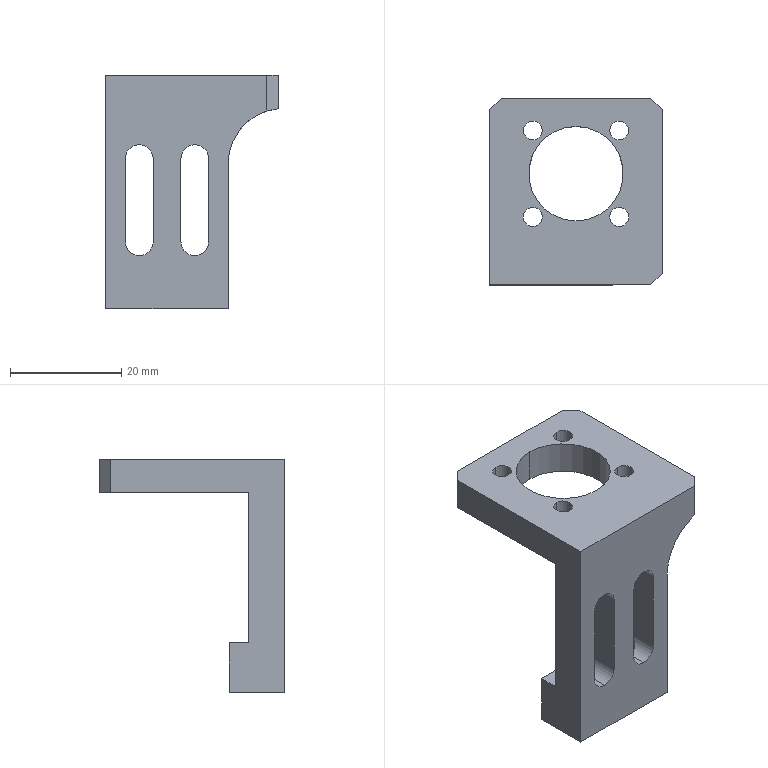Part | 1 solid | 39 faces | box 31 x 33.478 x 42 mm | volume 9262 mm3 | cylinder 21 | plane 18 | commonest cylinder face diameters 3.4 x8 5 x6 2.5 x4 17 x2 20 x1
STEP:
#1=CARTESIAN_POINT('',(7.778,9.339,0.));
#2=VERTEX_POINT('',#1);
#3=CARTESIAN_POINT('',(7.778,12.739,0.));
#4=VERTEX_POINT('',#3);
#5=CARTESIAN_POINT('',(7.778,11.039,0.));
#6=DIRECTION('',(0.,0.,-1.));
#7=DIRECTION('',(0.,1.,0.));
#8=AXIS2_PLACEMENT_3D('',#5,#6,#7);
#9=CIRCLE('',#8,1.7);
#10=EDGE_CURVE('',#2,#4,#9,.T.);
#11=ORIENTED_EDGE('',*,*,#10,.F.);
#12=CARTESIAN_POINT('',(7.778,9.339,-6.));
#13=VERTEX_POINT('',#12);
#14=CARTESIAN_POINT('',(7.778,9.339,-6.));
#15=DIRECTION('',(0.,0.,-1.));
#16=VECTOR('',#15,1000.);
#17=LINE('',#14,#16);
#18=EDGE_CURVE('',#13,#2,#17,.F.);
#19=ORIENTED_EDGE('',*,*,#18,.F.);
#20=CARTESIAN_POINT('',(7.778,12.739,-6.));
#21=VERTEX_POINT('',#20);
#22=CARTESIAN_POINT('',(7.778,11.039,-6.));
#23=DIRECTION('',(0.,0.,-1.));
#24=DIRECTION('',(0.,1.,0.));
#25=AXIS2_PLACEMENT_3D('',#22,#23,#24);
#26=CIRCLE('',#25,1.7);
#27=EDGE_CURVE('',#13,#21,#26,.T.);
#28=ORIENTED_EDGE('',*,*,#27,.T.);
#29=CARTESIAN_POINT('',(7.778,12.739,-6.));
#30=DIRECTION('',(0.,0.,-1.));
#31=VECTOR('',#30,1000.);
#32=LINE('',#29,#31);
#33=EDGE_CURVE('',#21,#4,#32,.F.);
#34=ORIENTED_EDGE('',*,*,#33,.T.);
#35=EDGE_LOOP('',(#11,#19,#28,#34));
#36=FACE_BOUND('',#35,.T.);
#37=CARTESIAN_POINT('',(7.778,11.039,-6.));
#38=DIRECTION('',(0.,0.,-1.));
#39=DIRECTION('',(0.,-1.,0.));
#40=AXIS2_PLACEMENT_3D('',#37,#38,#39);
#41=CYLINDRICAL_SURFACE('',#40,1.7);
#42=ADVANCED_FACE('',(#36),#41,.F.);
#43=CARTESIAN_POINT('',(7.778,-6.217,0.));
#44=VERTEX_POINT('',#43);
#45=CARTESIAN_POINT('',(7.778,-2.817,0.));
#46=VERTEX_POINT('',#45);
#47=CARTESIAN_POINT('',(7.778,-4.517,0.));
#48=DIRECTION('',(0.,0.,-1.));
#49=DIRECTION('',(0.,1.,0.));
#50=AXIS2_PLACEMENT_3D('',#47,#48,#49);
#51=CIRCLE('',#50,1.7);
#52=EDGE_CURVE('',#44,#46,#51,.T.);
#53=ORIENTED_EDGE('',*,*,#52,.F.);
#54=CARTESIAN_POINT('',(7.778,-6.217,-6.));
#55=VERTEX_POINT('',#54);
#56=CARTESIAN_POINT('',(7.778,-6.217,-6.));
#57=DIRECTION('',(0.,0.,-1.));
#58=VECTOR('',#57,1000.);
#59=LINE('',#56,#58);
#60=EDGE_CURVE('',#55,#44,#59,.F.);
#61=ORIENTED_EDGE('',*,*,#60,.F.);
#62=CARTESIAN_POINT('',(7.778,-2.817,-6.));
#63=VERTEX_POINT('',#62);
#64=CARTESIAN_POINT('',(7.778,-4.517,-6.));
#65=DIRECTION('',(0.,0.,-1.));
#66=DIRECTION('',(0.,1.,0.));
#67=AXIS2_PLACEMENT_3D('',#64,#65,#66);
#68=CIRCLE('',#67,1.7);
#69=EDGE_CURVE('',#55,#63,#68,.T.);
#70=ORIENTED_EDGE('',*,*,#69,.T.);
#71=CARTESIAN_POINT('',(7.778,-2.817,-6.));
#72=DIRECTION('',(0.,0.,-1.));
#73=VECTOR('',#72,1000.);
#74=LINE('',#71,#73);
#75=EDGE_CURVE('',#63,#46,#74,.F.);
#76=ORIENTED_EDGE('',*,*,#75,.T.);
#77=EDGE_LOOP('',(#53,#61,#70,#76));
#78=FACE_BOUND('',#77,.T.);
#79=CARTESIAN_POINT('',(7.778,-4.517,-6.));
#80=DIRECTION('',(0.,0.,-1.));
#81=DIRECTION('',(0.,-1.,0.));
#82=AXIS2_PLACEMENT_3D('',#79,#80,#81);
#83=CYLINDRICAL_SURFACE('',#82,1.7);
#84=ADVANCED_FACE('',(#78),#83,.F.);
#85=CARTESIAN_POINT('',(-7.778,9.339,0.));
#86=VERTEX_POINT('',#85);
#87=CARTESIAN_POINT('',(-7.778,12.739,0.));
#88=VERTEX_POINT('',#87);
#89=CARTESIAN_POINT('',(-7.778,11.039,0.));
#90=DIRECTION('',(0.,0.,-1.));
#91=DIRECTION('',(0.,1.,0.));
#92=AXIS2_PLACEMENT_3D('',#89,#90,#91);
#93=CIRCLE('',#92,1.7);
#94=EDGE_CURVE('',#86,#88,#93,.T.);
#95=ORIENTED_EDGE('',*,*,#94,.F.);
#96=CARTESIAN_POINT('',(-7.778,9.339,-6.));
#97=VERTEX_POINT('',#96);
#98=CARTESIAN_POINT('',(-7.778,9.339,-6.));
#99=DIRECTION('',(0.,0.,-1.));
#100=VECTOR('',#99,1000.);
#101=LINE('',#98,#100);
#102=EDGE_CURVE('',#97,#86,#101,.F.);
#103=ORIENTED_EDGE('',*,*,#102,.F.);
#104=CARTESIAN_POINT('',(-7.778,12.739,-6.));
#105=VERTEX_POINT('',#104);
#106=CARTESIAN_POINT('',(-7.778,11.039,-6.));
#107=DIRECTION('',(0.,0.,-1.));
#108=DIRECTION('',(0.,1.,0.));
#109=AXIS2_PLACEMENT_3D('',#106,#107,#108);
#110=CIRCLE('',#109,1.7);
#111=EDGE_CURVE('',#97,#105,#110,.T.);
#112=ORIENTED_EDGE('',*,*,#111,.T.);
#113=CARTESIAN_POINT('',(-7.778,12.739,-6.));
#114=DIRECTION('',(0.,0.,-1.));
#115=VECTOR('',#114,1000.);
#116=LINE('',#113,#115);
#117=EDGE_CURVE('',#105,#88,#116,.F.);
#118=ORIENTED_EDGE('',*,*,#117,.T.);
#119=EDGE_LOOP('',(#95,#103,#112,#118));
#120=FACE_BOUND('',#119,.T.);
#121=CARTESIAN_POINT('',(-7.778,11.039,-6.));
#122=DIRECTION('',(0.,0.,-1.));
#123=DIRECTION('',(0.,-1.,0.));
#124=AXIS2_PLACEMENT_3D('',#121,#122,#123);
#125=CYLINDRICAL_SURFACE('',#124,1.7);
#126=ADVANCED_FACE('',(#120),#125,.F.);
#127=CARTESIAN_POINT('',(-7.778,-6.217,0.));
#128=VERTEX_POINT('',#127);
#129=CARTESIAN_POINT('',(-7.778,-2.817,0.));
#130=VERTEX_POINT('',#129);
#131=CARTESIAN_POINT('',(-7.778,-4.517,0.));
#132=DIRECTION('',(0.,0.,-1.));
#133=DIRECTION('',(0.,1.,0.));
#134=AXIS2_PLACEMENT_3D('',#131,#132,#133);
#135=CIRCLE('',#134,1.7);
#136=EDGE_CURVE('',#128,#130,#135,.T.);
#137=ORIENTED_EDGE('',*,*,#136,.F.);
#138=CARTESIAN_POINT('',(-7.778,-6.217,-6.));
#139=VERTEX_POINT('',#138);
#140=CARTESIAN_POINT('',(-7.778,-6.217,-6.));
#141=DIRECTION('',(0.,0.,-1.));
#142=VECTOR('',#141,1000.);
#143=LINE('',#140,#142);
#144=EDGE_CURVE('',#139,#128,#143,.F.);
#145=ORIENTED_EDGE('',*,*,#144,.F.);
#146=CARTESIAN_POINT('',(-7.778,-2.817,-6.));
#147=VERTEX_POINT('',#146);
#148=CARTESIAN_POINT('',(-7.778,-4.517,-6.));
#149=DIRECTION('',(0.,0.,-1.));
#150=DIRECTION('',(0.,1.,0.));
#151=AXIS2_PLACEMENT_3D('',#148,#149,#150);
#152=CIRCLE('',#151,1.7);
#153=EDGE_CURVE('',#139,#147,#152,.T.);
#154=ORIENTED_EDGE('',*,*,#153,.T.);
#155=CARTESIAN_POINT('',(-7.778,-2.817,-6.));
#156=DIRECTION('',(0.,0.,-1.));
#157=VECTOR('',#156,1000.);
#158=LINE('',#155,#157);
#159=EDGE_CURVE('',#147,#130,#158,.F.);
#160=ORIENTED_EDGE('',*,*,#159,.T.);
#161=EDGE_LOOP('',(#137,#145,#154,#160));
#162=FACE_BOUND('',#161,.T.);
#163=CARTESIAN_POINT('',(-7.778,-4.517,-6.));
#164=DIRECTION('',(0.,0.,-1.));
#165=DIRECTION('',(0.,-1.,0.));
#166=AXIS2_PLACEMENT_3D('',#163,#164,#165);
#167=CYLINDRICAL_SURFACE('',#166,1.7);
#168=ADVANCED_FACE('',(#162),#167,.F.);
#169=CARTESIAN_POINT('',(0.,-5.239,-6.));
#170=VERTEX_POINT('',#169);
#171=CARTESIAN_POINT('',(0.,11.761,-6.));
#172=VERTEX_POINT('',#171);
#173=CARTESIAN_POINT('',(0.,3.261,-6.));
#174=DIRECTION('',(0.,0.,-1.));
#175=DIRECTION('',(0.,1.,0.));
#176=AXIS2_PLACEMENT_3D('',#173,#174,#175);
#177=CIRCLE('',#176,8.5);
#178=EDGE_CURVE('',#170,#172,#177,.T.);
#179=ORIENTED_EDGE('',*,*,#178,.T.);
#180=CARTESIAN_POINT('',(0.,11.761,0.));
#181=VERTEX_POINT('',#180);
#182=CARTESIAN_POINT('',(0.,11.761,-42.));
#183=DIRECTION('',(0.,0.,1.));
#184=VECTOR('',#183,1000.);
#185=LINE('',#182,#184);
#186=EDGE_CURVE('',#181,#172,#185,.F.);
#187=ORIENTED_EDGE('',*,*,#186,.F.);
#188=CARTESIAN_POINT('',(0.,-5.239,0.));
#189=VERTEX_POINT('',#188);
#190=CARTESIAN_POINT('',(0.,3.261,0.));
#191=DIRECTION('',(0.,0.,1.));
#192=DIRECTION('',(0.,-1.,0.));
#193=AXIS2_PLACEMENT_3D('',#190,#191,#192);
#194=CIRCLE('',#193,8.5);
#195=EDGE_CURVE('',#181,#189,#194,.T.);
#196=ORIENTED_EDGE('',*,*,#195,.T.);
#197=CARTESIAN_POINT('',(0.,-5.239,-42.));
#198=DIRECTION('',(0.,0.,1.));
#199=VECTOR('',#198,1000.);
#200=LINE('',#197,#199);
#201=EDGE_CURVE('',#189,#170,#200,.F.);
#202=ORIENTED_EDGE('',*,*,#201,.T.);
#203=EDGE_LOOP('',(#179,#187,#196,#202));
#204=FACE_BOUND('',#203,.T.);
#205=CARTESIAN_POINT('',(0.,3.261,-42.));
#206=DIRECTION('',(0.,0.,1.));
#207=DIRECTION('',(0.,1.,0.));
#208=AXIS2_PLACEMENT_3D('',#205,#206,#207);
#209=CYLINDRICAL_SURFACE('',#208,8.5);
#210=ADVANCED_FACE('',(#204),#209,.F.);
#211=CARTESIAN_POINT('',(-7.,-10.239,-30.));
#212=VERTEX_POINT('',#211);
#213=CARTESIAN_POINT('',(-9.5,-10.239,-32.5));
#214=VERTEX_POINT('',#213);
#215=CARTESIAN_POINT('',(-9.5,-10.239,-30.));
#216=DIRECTION('',(0.,1.,0.));
#217=DIRECTION('',(0.,0.,-1.));
#218=AXIS2_PLACEMENT_3D('',#215,#216,#217);
#219=CIRCLE('',#218,2.5);
#220=EDGE_CURVE('',#212,#214,#219,.T.);
#221=ORIENTED_EDGE('',*,*,#220,.T.);
#222=CARTESIAN_POINT('',(-9.5,-10.989,-32.5));
#223=VERTEX_POINT('',#222);
#224=CARTESIAN_POINT('',(-9.5,25.261,-32.5));
#225=DIRECTION('',(0.,-1.,0.));
#226=VECTOR('',#225,1000.);
#227=LINE('',#224,#226);
#228=EDGE_CURVE('',#214,#223,#227,.T.);
#229=ORIENTED_EDGE('',*,*,#228,.T.);
#230=CARTESIAN_POINT('',(-9.5,-12.489,-32.5));
#231=VERTEX_POINT('',#230);
#232=CARTESIAN_POINT('',(-9.5,-12.489,-32.5));
#233=CARTESIAN_POINT('',(-9.175,-12.056,-32.5));
#234=CARTESIAN_POINT('',(-9.175,-11.422,-32.5));
#235=CARTESIAN_POINT('',(-9.5,-10.989,-32.5));
#236=B_SPLINE_CURVE_WITH_KNOTS('',3,(#232,#233,#234,#235),.UNSPECIFIED.,.F.,.F.,(4,4),(0.,0.0016),.UNSPECIFIED.);
#237=EDGE_CURVE('',#231,#223,#236,.T.);
#238=ORIENTED_EDGE('',*,*,#237,.F.);
#239=CARTESIAN_POINT('',(-9.5,-16.739,-32.5));
#240=VERTEX_POINT('',#239);
#241=CARTESIAN_POINT('',(-9.5,25.261,-32.5));
#242=DIRECTION('',(0.,-1.,0.));
#243=VECTOR('',#242,1000.);
#244=LINE('',#241,#243);
#245=EDGE_CURVE('',#231,#240,#244,.T.);
#246=ORIENTED_EDGE('',*,*,#245,.T.);
#247=CARTESIAN_POINT('',(-7.,-16.739,-30.));
#248=VERTEX_POINT('',#247);
#249=CARTESIAN_POINT('',(-9.5,-16.739,-30.));
#250=DIRECTION('',(0.,-1.,0.));
#251=DIRECTION('',(0.,0.,-1.));
#252=AXIS2_PLACEMENT_3D('',#249,#250,#251);
#253=CIRCLE('',#252,2.5);
#254=EDGE_CURVE('',#240,#248,#253,.T.);
#255=ORIENTED_EDGE('',*,*,#254,.T.);
#256=CARTESIAN_POINT('',(-7.,25.261,-30.));
#257=DIRECTION('',(0.,-1.,0.));
#258=VECTOR('',#257,1000.);
#259=LINE('',#256,#258);
#260=EDGE_CURVE('',#212,#248,#259,.T.);
#261=ORIENTED_EDGE('',*,*,#260,.F.);
#262=EDGE_LOOP('',(#221,#229,#238,#246,#255,#261));
#263=FACE_BOUND('',#262,.T.);
#264=CARTESIAN_POINT('',(-9.5,25.261,-30.));
#265=DIRECTION('',(0.,-1.,0.));
#266=DIRECTION('',(0.,0.,1.));
#267=AXIS2_PLACEMENT_3D('',#264,#265,#266);
#268=CYLINDRICAL_SURFACE('',#267,2.5);
#269=ADVANCED_FACE('',(#263),#268,.F.);
#270=CARTESIAN_POINT('',(3.,-10.239,-30.));
#271=VERTEX_POINT('',#270);
#272=CARTESIAN_POINT('',(0.5,-10.239,-32.5));
#273=VERTEX_POINT('',#272);
#274=CARTESIAN_POINT('',(0.5,-10.239,-30.));
#275=DIRECTION('',(0.,1.,0.));
#276=DIRECTION('',(0.,0.,-1.));
#277=AXIS2_PLACEMENT_3D('',#274,#275,#276);
#278=CIRCLE('',#277,2.5);
#279=EDGE_CURVE('',#271,#273,#278,.T.);
#280=ORIENTED_EDGE('',*,*,#279,.T.);
#281=CARTESIAN_POINT('',(0.5,-10.989,-32.5));
#282=VERTEX_POINT('',#281);
#283=CARTESIAN_POINT('',(0.5,25.261,-32.5));
#284=DIRECTION('',(0.,-1.,0.));
#285=VECTOR('',#284,1000.);
#286=LINE('',#283,#285);
#287=EDGE_CURVE('',#273,#282,#286,.T.);
#288=ORIENTED_EDGE('',*,*,#287,.T.);
#289=CARTESIAN_POINT('',(1.5,-10.489,-32.291));
#290=VERTEX_POINT('',#289);
#291=CARTESIAN_POINT('',(1.5,-10.489,-32.291));
#292=CARTESIAN_POINT('',(1.134,-10.489,-32.451));
#293=CARTESIAN_POINT('',(0.7396,-10.67,-32.5));
#294=CARTESIAN_POINT('',(0.5,-10.989,-32.5));
#295=B_SPLINE_CURVE_WITH_KNOTS('',3,(#291,#292,#293,#294),.UNSPECIFIED.,.F.,.F.,(4,4),(0.,0.001181),.UNSPECIFIED.);
#296=EDGE_CURVE('',#290,#282,#295,.T.);
#297=ORIENTED_EDGE('',*,*,#296,.F.);
#298=CARTESIAN_POINT('',(1.5,-12.989,-32.291));
#299=VERTEX_POINT('',#298);
#300=CARTESIAN_POINT('',(1.5,-12.989,-32.291));
#301=CARTESIAN_POINT('',(1.859,-12.989,-32.134));
#302=CARTESIAN_POINT('',(2.307,-12.765,-31.78));
#303=CARTESIAN_POINT('',(2.657,-12.293,-31.285));
#304=CARTESIAN_POINT('',(2.796,-11.741,-30.992));
#305=CARTESIAN_POINT('',(2.658,-11.187,-31.284));
#306=CARTESIAN_POINT('',(2.309,-10.714,-31.779));
#307=CARTESIAN_POINT('',(1.859,-10.489,-32.135));
#308=CARTESIAN_POINT('',(1.5,-10.489,-32.291));
#309=B_SPLINE_CURVE_WITH_KNOTS('',3,(#300,#301,#302,#303,#304,#305,#306,#307,#308),.UNSPECIFIED.,.F.,.F.,(4,1,1,1,1,1,4),(0.,0.001157,0.001735,0.002314,0.002892,0.003471,0.004627),.UNSPECIFIED.);
#310=EDGE_CURVE('',#299,#290,#309,.T.);
#311=ORIENTED_EDGE('',*,*,#310,.F.);
#312=CARTESIAN_POINT('',(0.5,-12.489,-32.5));
#313=VERTEX_POINT('',#312);
#314=CARTESIAN_POINT('',(0.5,-12.489,-32.5));
#315=CARTESIAN_POINT('',(0.7395,-12.808,-32.5));
#316=CARTESIAN_POINT('',(1.134,-12.989,-32.451));
#317=CARTESIAN_POINT('',(1.5,-12.989,-32.291));
#318=B_SPLINE_CURVE_WITH_KNOTS('',3,(#314,#315,#316,#317),.UNSPECIFIED.,.F.,.F.,(4,4),(0.,0.001181),.UNSPECIFIED.);
#319=EDGE_CURVE('',#313,#299,#318,.T.);
#320=ORIENTED_EDGE('',*,*,#319,.F.);
#321=CARTESIAN_POINT('',(0.5,-16.739,-32.5));
#322=VERTEX_POINT('',#321);
#323=CARTESIAN_POINT('',(0.5,25.261,-32.5));
#324=DIRECTION('',(0.,-1.,0.));
#325=VECTOR('',#324,1000.);
#326=LINE('',#323,#325);
#327=EDGE_CURVE('',#313,#322,#326,.T.);
#328=ORIENTED_EDGE('',*,*,#327,.T.);
#329=CARTESIAN_POINT('',(3.,-16.739,-30.));
#330=VERTEX_POINT('',#329);
#331=CARTESIAN_POINT('',(0.5,-16.739,-30.));
#332=DIRECTION('',(0.,-1.,0.));
#333=DIRECTION('',(0.,0.,-1.));
#334=AXIS2_PLACEMENT_3D('',#331,#332,#333);
#335=CIRCLE('',#334,2.5);
#336=EDGE_CURVE('',#322,#330,#335,.T.);
#337=ORIENTED_EDGE('',*,*,#336,.T.);
#338=CARTESIAN_POINT('',(3.,25.261,-30.));
#339=DIRECTION('',(0.,-1.,0.));
#340=VECTOR('',#339,1000.);
#341=LINE('',#338,#340);
#342=EDGE_CURVE('',#271,#330,#341,.T.);
#343=ORIENTED_EDGE('',*,*,#342,.F.);
#344=EDGE_LOOP('',(#280,#288,#297,#311,#320,#328,#337,#343));
#345=FACE_BOUND('',#344,.T.);
#346=CARTESIAN_POINT('',(0.5,25.261,-30.));
#347=DIRECTION('',(0.,-1.,0.));
#348=DIRECTION('',(0.,0.,1.));
#349=AXIS2_PLACEMENT_3D('',#346,#347,#348);
#350=CYLINDRICAL_SURFACE('',#349,2.5);
#351=ADVANCED_FACE('',(#345),#350,.F.);
#352=ORIENTED_EDGE('',*,*,#296,.T.);
#353=CARTESIAN_POINT('',(0.5,-10.989,-32.5));
#354=CARTESIAN_POINT('',(0.1753,-11.422,-32.5));
#355=CARTESIAN_POINT('',(0.1753,-12.056,-32.5));
#356=CARTESIAN_POINT('',(0.5,-12.489,-32.5));
#357=B_SPLINE_CURVE_WITH_KNOTS('',3,(#353,#354,#355,#356),.UNSPECIFIED.,.F.,.F.,(4,4),(0.,0.0016),.UNSPECIFIED.);
#358=EDGE_CURVE('',#282,#313,#357,.T.);
#359=ORIENTED_EDGE('',*,*,#358,.T.);
#360=ORIENTED_EDGE('',*,*,#319,.T.);
#361=CARTESIAN_POINT('',(1.5,-12.989,-42.));
#362=VERTEX_POINT('',#361);
#363=CARTESIAN_POINT('',(1.5,-12.989,-42.));
#364=DIRECTION('',(0.,0.,-1.));
#365=VECTOR('',#364,1000.);
#366=LINE('',#363,#365);
#367=EDGE_CURVE('',#362,#299,#366,.F.);
#368=ORIENTED_EDGE('',*,*,#367,.F.);
#369=CARTESIAN_POINT('',(1.5,-10.489,-42.));
#370=VERTEX_POINT('',#369);
#371=CARTESIAN_POINT('',(1.5,-11.739,-42.));
#372=DIRECTION('',(0.,0.,-1.));
#373=DIRECTION('',(0.,1.,0.));
#374=AXIS2_PLACEMENT_3D('',#371,#372,#373);
#375=CIRCLE('',#374,1.25);
#376=EDGE_CURVE('',#362,#370,#375,.T.);
#377=ORIENTED_EDGE('',*,*,#376,.T.);
#378=CARTESIAN_POINT('',(1.5,-10.489,-42.));
#379=DIRECTION('',(0.,0.,-1.));
#380=VECTOR('',#379,1000.);
#381=LINE('',#378,#380);
#382=EDGE_CURVE('',#370,#290,#381,.F.);
#383=ORIENTED_EDGE('',*,*,#382,.T.);
#384=EDGE_LOOP('',(#352,#359,#360,#368,#377,#383));
#385=FACE_BOUND('',#384,.T.);
#386=CARTESIAN_POINT('',(1.5,-11.739,-42.));
#387=DIRECTION('',(0.,0.,-1.));
#388=DIRECTION('',(0.,-1.,0.));
#389=AXIS2_PLACEMENT_3D('',#386,#387,#388);
#390=CYLINDRICAL_SURFACE('',#389,1.25);
#391=ADVANCED_FACE('',(#385),#390,.F.);
#392=CARTESIAN_POINT('',(-10.5,-10.489,-32.291));
#393=VERTEX_POINT('',#392);
#394=CARTESIAN_POINT('',(-10.5,-12.989,-32.291));
#395=VERTEX_POINT('',#394);
#396=CARTESIAN_POINT('',(-10.5,-10.489,-32.291));
#397=CARTESIAN_POINT('',(-10.859,-10.489,-32.134));
#398=CARTESIAN_POINT('',(-11.307,-10.713,-31.78));
#399=CARTESIAN_POINT('',(-11.657,-11.185,-31.285));
#400=CARTESIAN_POINT('',(-11.796,-11.738,-30.992));
#401=CARTESIAN_POINT('',(-11.658,-12.291,-31.284));
#402=CARTESIAN_POINT('',(-11.309,-12.764,-31.779));
#403=CARTESIAN_POINT('',(-10.859,-12.989,-32.135));
#404=CARTESIAN_POINT('',(-10.5,-12.989,-32.291));
#405=B_SPLINE_CURVE_WITH_KNOTS('',3,(#396,#397,#398,#399,#400,#401,#402,#403,#404),.UNSPECIFIED.,.F.,.F.,(4,1,1,1,1,1,4),(0.,0.001157,0.001735,0.002314,0.002892,0.003471,0.004627),.UNSPECIFIED.);
#406=EDGE_CURVE('',#393,#395,#405,.T.);
#407=ORIENTED_EDGE('',*,*,#406,.T.);
#408=CARTESIAN_POINT('',(-10.5,-12.989,-42.));
#409=VERTEX_POINT('',#408);
#410=CARTESIAN_POINT('',(-10.5,-12.989,-42.));
#411=DIRECTION('',(0.,0.,-1.));
#412=VECTOR('',#411,1000.);
#413=LINE('',#410,#412);
#414=EDGE_CURVE('',#409,#395,#413,.F.);
#415=ORIENTED_EDGE('',*,*,#414,.F.);
#416=CARTESIAN_POINT('',(-10.5,-10.489,-42.));
#417=VERTEX_POINT('',#416);
#418=CARTESIAN_POINT('',(-10.5,-11.739,-42.));
#419=DIRECTION('',(0.,0.,-1.));
#420=DIRECTION('',(0.,1.,0.));
#421=AXIS2_PLACEMENT_3D('',#418,#419,#420);
#422=CIRCLE('',#421,1.25);
#423=EDGE_CURVE('',#409,#417,#422,.T.);
#424=ORIENTED_EDGE('',*,*,#423,.T.);
#425=CARTESIAN_POINT('',(-10.5,-10.489,-42.));
#426=DIRECTION('',(0.,0.,-1.));
#427=VECTOR('',#426,1000.);
#428=LINE('',#425,#427);
#429=EDGE_CURVE('',#417,#393,#428,.F.);
#430=ORIENTED_EDGE('',*,*,#429,.T.);
#431=EDGE_LOOP('',(#407,#415,#424,#430));
#432=FACE_BOUND('',#431,.T.);
#433=CARTESIAN_POINT('',(-10.5,-11.739,-42.));
#434=DIRECTION('',(0.,0.,-1.));
#435=DIRECTION('',(0.,-1.,0.));
#436=AXIS2_PLACEMENT_3D('',#433,#434,#435);
#437=CYLINDRICAL_SURFACE('',#436,1.25);
#438=ADVANCED_FACE('',(#432),#437,.F.);
#439=CARTESIAN_POINT('',(15.5,-14.739,0.));
#440=VERTEX_POINT('',#439);
#441=CARTESIAN_POINT('',(15.5,14.739,0.));
#442=VERTEX_POINT('',#441);
#443=CARTESIAN_POINT('',(15.5,25.261,0.));
#444=DIRECTION('',(0.,1.,0.));
#445=VECTOR('',#444,1000.);
#446=LINE('',#443,#445);
#447=EDGE_CURVE('',#440,#442,#446,.T.);
#448=ORIENTED_EDGE('',*,*,#447,.F.);
#449=CARTESIAN_POINT('',(15.5,-14.739,-6.));
#450=VERTEX_POINT('',#449);
#451=CARTESIAN_POINT('',(15.5,-14.739,-6.));
#452=DIRECTION('',(0.,0.,-1.));
#453=VECTOR('',#452,1000.);
#454=LINE('',#451,#453);
#455=EDGE_CURVE('',#440,#450,#454,.T.);
#456=ORIENTED_EDGE('',*,*,#455,.T.);
#457=CARTESIAN_POINT('',(15.5,-10.239,-6.));
#458=VERTEX_POINT('',#457);
#459=CARTESIAN_POINT('',(15.5,25.261,-6.));
#460=DIRECTION('',(0.,1.,0.));
#461=VECTOR('',#460,1000.);
#462=LINE('',#459,#461);
#463=EDGE_CURVE('',#450,#458,#462,.T.);
#464=ORIENTED_EDGE('',*,*,#463,.T.);
#465=CARTESIAN_POINT('',(15.5,14.739,-6.));
#466=VERTEX_POINT('',#465);
#467=CARTESIAN_POINT('',(15.5,25.261,-6.));
#468=DIRECTION('',(0.,1.,0.));
#469=VECTOR('',#468,1000.);
#470=LINE('',#467,#469);
#471=EDGE_CURVE('',#458,#466,#470,.T.);
#472=ORIENTED_EDGE('',*,*,#471,.T.);
#473=CARTESIAN_POINT('',(15.5,14.739,0.));
#474=DIRECTION('',(0.,0.,1.));
#475=VECTOR('',#474,1000.);
#476=LINE('',#473,#475);
#477=EDGE_CURVE('',#466,#442,#476,.T.);
#478=ORIENTED_EDGE('',*,*,#477,.T.);
#479=EDGE_LOOP('',(#448,#456,#464,#472,#478));
#480=FACE_BOUND('',#479,.T.);
#481=CARTESIAN_POINT('',(15.5,25.261,0.));
#482=DIRECTION('',(-1.,0.,0.));
#483=DIRECTION('',(0.,0.,1.));
#484=AXIS2_PLACEMENT_3D('',#481,#482,#483);
#485=PLANE('',#484);
#486=ADVANCED_FACE('',(#480),#485,.F.);
#487=CARTESIAN_POINT('',(-15.5,14.739,0.));
#488=VERTEX_POINT('',#487);
#489=CARTESIAN_POINT('',(-15.5,-16.739,0.));
#490=VERTEX_POINT('',#489);
#491=CARTESIAN_POINT('',(-15.5,25.261,0.));
#492=DIRECTION('',(0.,-1.,0.));
#493=VECTOR('',#492,1000.);
#494=LINE('',#491,#493);
#495=EDGE_CURVE('',#488,#490,#494,.T.);
#496=ORIENTED_EDGE('',*,*,#495,.F.);
#497=CARTESIAN_POINT('',(-15.5,14.739,-6.));
#498=VERTEX_POINT('',#497);
#499=CARTESIAN_POINT('',(-15.5,14.739,0.));
#500=DIRECTION('',(0.,0.,-1.));
#501=VECTOR('',#500,1000.);
#502=LINE('',#499,#501);
#503=EDGE_CURVE('',#488,#498,#502,.T.);
#504=ORIENTED_EDGE('',*,*,#503,.T.);
#505=CARTESIAN_POINT('',(-15.5,-10.239,-6.));
#506=VERTEX_POINT('',#505);
#507=CARTESIAN_POINT('',(-15.5,25.261,-6.));
#508=DIRECTION('',(0.,-1.,0.));
#509=VECTOR('',#508,1000.);
#510=LINE('',#507,#509);
#511=EDGE_CURVE('',#498,#506,#510,.T.);
#512=ORIENTED_EDGE('',*,*,#511,.T.);
#513=CARTESIAN_POINT('',(-15.5,-10.239,-33.));
#514=VERTEX_POINT('',#513);
#515=CARTESIAN_POINT('',(-15.5,-10.239,-6.));
#516=DIRECTION('',(0.,0.,1.));
#517=VECTOR('',#516,1000.);
#518=LINE('',#515,#517);
#519=EDGE_CURVE('',#514,#506,#518,.T.);
#520=ORIENTED_EDGE('',*,*,#519,.F.);
#521=CARTESIAN_POINT('',(-15.5,-6.739,-33.));
#522=VERTEX_POINT('',#521);
#523=CARTESIAN_POINT('',(-15.5,-6.739,-33.));
#524=DIRECTION('',(0.,-1.,0.));
#525=VECTOR('',#524,1000.);
#526=LINE('',#523,#525);
#527=EDGE_CURVE('',#522,#514,#526,.T.);
#528=ORIENTED_EDGE('',*,*,#527,.F.);
#529=CARTESIAN_POINT('',(-15.5,-6.739,-42.));
#530=VERTEX_POINT('',#529);
#531=CARTESIAN_POINT('',(-15.5,-6.739,-42.));
#532=DIRECTION('',(0.,0.,1.));
#533=VECTOR('',#532,1000.);
#534=LINE('',#531,#533);
#535=EDGE_CURVE('',#530,#522,#534,.T.);
#536=ORIENTED_EDGE('',*,*,#535,.F.);
#537=CARTESIAN_POINT('',(-15.5,-16.739,-42.));
#538=VERTEX_POINT('',#537);
#539=CARTESIAN_POINT('',(-15.5,-16.739,-42.));
#540=DIRECTION('',(0.,1.,0.));
#541=VECTOR('',#540,1000.);
#542=LINE('',#539,#541);
#543=EDGE_CURVE('',#538,#530,#542,.T.);
#544=ORIENTED_EDGE('',*,*,#543,.F.);
#545=CARTESIAN_POINT('',(-15.5,-16.739,0.));
#546=DIRECTION('',(0.,0.,-1.));
#547=VECTOR('',#546,1000.);
#548=LINE('',#545,#547);
#549=EDGE_CURVE('',#490,#538,#548,.T.);
#550=ORIENTED_EDGE('',*,*,#549,.F.);
#551=EDGE_LOOP('',(#496,#504,#512,#520,#528,#536,#544,#550));
#552=FACE_BOUND('',#551,.T.);
#553=CARTESIAN_POINT('',(-15.5,25.261,0.));
#554=DIRECTION('',(1.,0.,0.));
#555=DIRECTION('',(0.,0.,-1.));
#556=AXIS2_PLACEMENT_3D('',#553,#554,#555);
#557=PLANE('',#556);
#558=ADVANCED_FACE('',(#552),#557,.F.);
#559=CARTESIAN_POINT('',(7.778,11.039,0.));
#560=DIRECTION('',(0.,0.,-1.));
#561=DIRECTION('',(0.,1.,0.));
#562=AXIS2_PLACEMENT_3D('',#559,#560,#561);
#563=CIRCLE('',#562,1.7);
#564=EDGE_CURVE('',#4,#2,#563,.T.);
#565=ORIENTED_EDGE('',*,*,#564,.T.);
#566=ORIENTED_EDGE('',*,*,#10,.T.);
#567=EDGE_LOOP('',(#565,#566));
#568=FACE_BOUND('',#567,.T.);
#569=CARTESIAN_POINT('',(7.778,-4.517,0.));
#570=DIRECTION('',(0.,0.,-1.));
#571=DIRECTION('',(0.,1.,0.));
#572=AXIS2_PLACEMENT_3D('',#569,#570,#571);
#573=CIRCLE('',#572,1.7);
#574=EDGE_CURVE('',#46,#44,#573,.T.);
#575=ORIENTED_EDGE('',*,*,#574,.T.);
#576=ORIENTED_EDGE('',*,*,#52,.T.);
#577=EDGE_LOOP('',(#575,#576));
#578=FACE_BOUND('',#577,.T.);
#579=CARTESIAN_POINT('',(-7.778,11.039,0.));
#580=DIRECTION('',(0.,0.,-1.));
#581=DIRECTION('',(0.,1.,0.));
#582=AXIS2_PLACEMENT_3D('',#579,#580,#581);
#583=CIRCLE('',#582,1.7);
#584=EDGE_CURVE('',#88,#86,#583,.T.);
#585=ORIENTED_EDGE('',*,*,#584,.T.);
#586=ORIENTED_EDGE('',*,*,#94,.T.);
#587=EDGE_LOOP('',(#585,#586));
#588=FACE_BOUND('',#587,.T.);
#589=CARTESIAN_POINT('',(-7.778,-4.517,0.));
#590=DIRECTION('',(0.,0.,-1.));
#591=DIRECTION('',(0.,1.,0.));
#592=AXIS2_PLACEMENT_3D('',#589,#590,#591);
#593=CIRCLE('',#592,1.7);
#594=EDGE_CURVE('',#130,#128,#593,.T.);
#595=ORIENTED_EDGE('',*,*,#594,.T.);
#596=ORIENTED_EDGE('',*,*,#136,.T.);
#597=EDGE_LOOP('',(#595,#596));
#598=FACE_BOUND('',#597,.T.);
#599=CARTESIAN_POINT('',(0.,3.261,0.));
#600=DIRECTION('',(0.,0.,1.));
#601=DIRECTION('',(0.,-1.,0.));
#602=AXIS2_PLACEMENT_3D('',#599,#600,#601);
#603=CIRCLE('',#602,8.5);
#604=EDGE_CURVE('',#189,#181,#603,.T.);
#605=ORIENTED_EDGE('',*,*,#604,.F.);
#606=ORIENTED_EDGE('',*,*,#195,.F.);
#607=EDGE_LOOP('',(#605,#606));
#608=FACE_BOUND('',#607,.T.);
#609=CARTESIAN_POINT('',(13.5,-16.739,0.));
#610=VERTEX_POINT('',#609);
#611=CARTESIAN_POINT('',(15.5,-16.739,0.));
#612=DIRECTION('',(-1.,0.,0.));
#613=VECTOR('',#612,1000.);
#614=LINE('',#611,#613);
#615=EDGE_CURVE('',#610,#490,#614,.T.);
#616=ORIENTED_EDGE('',*,*,#615,.F.);
#617=CARTESIAN_POINT('',(13.5,-16.739,0.));
#618=DIRECTION('',(0.7071,0.7071,0.));
#619=VECTOR('',#618,1000.);
#620=LINE('',#617,#619);
#621=EDGE_CURVE('',#610,#440,#620,.T.);
#622=ORIENTED_EDGE('',*,*,#621,.T.);
#623=ORIENTED_EDGE('',*,*,#447,.T.);
#624=CARTESIAN_POINT('',(13.5,16.739,0.));
#625=VERTEX_POINT('',#624);
#626=CARTESIAN_POINT('',(13.5,16.739,0.));
#627=DIRECTION('',(-0.7071,0.7071,0.));
#628=VECTOR('',#627,1000.);
#629=LINE('',#626,#628);
#630=EDGE_CURVE('',#442,#625,#629,.T.);
#631=ORIENTED_EDGE('',*,*,#630,.T.);
#632=CARTESIAN_POINT('',(-13.5,16.739,0.));
#633=VERTEX_POINT('',#632);
#634=CARTESIAN_POINT('',(15.5,16.739,0.));
#635=DIRECTION('',(-1.,0.,0.));
#636=VECTOR('',#635,1000.);
#637=LINE('',#634,#636);
#638=EDGE_CURVE('',#625,#633,#637,.T.);
#639=ORIENTED_EDGE('',*,*,#638,.T.);
#640=CARTESIAN_POINT('',(-15.5,14.739,0.));
#641=DIRECTION('',(-0.7071,-0.7071,0.));
#642=VECTOR('',#641,1000.);
#643=LINE('',#640,#642);
#644=EDGE_CURVE('',#633,#488,#643,.T.);
#645=ORIENTED_EDGE('',*,*,#644,.T.);
#646=ORIENTED_EDGE('',*,*,#495,.T.);
#647=EDGE_LOOP('',(#616,#622,#623,#631,#639,#645,#646));
#648=FACE_BOUND('',#647,.T.);
#649=CARTESIAN_POINT('',(0.,9.261,0.));
#650=DIRECTION('',(0.,0.,-1.));
#651=DIRECTION('',(0.,-1.,0.));
#652=AXIS2_PLACEMENT_3D('',#649,#650,#651);
#653=PLANE('',#652);
#654=ADVANCED_FACE('',(#568,#578,#588,#598,#608,#648),#653,.F.);
#655=CARTESIAN_POINT('',(13.5,16.739,-6.));
#656=VERTEX_POINT('',#655);
#657=CARTESIAN_POINT('',(-13.5,16.739,-6.));
#658=VERTEX_POINT('',#657);
#659=CARTESIAN_POINT('',(0.,16.739,-6.));
#660=DIRECTION('',(-1.,0.,0.));
#661=VECTOR('',#660,1000.);
#662=LINE('',#659,#661);
#663=EDGE_CURVE('',#656,#658,#662,.T.);
#664=ORIENTED_EDGE('',*,*,#663,.F.);
#665=CARTESIAN_POINT('',(10.489,19.75,-6.));
#666=DIRECTION('',(0.7071,-0.7071,0.));
#667=VECTOR('',#666,1000.);
#668=LINE('',#665,#667);
#669=EDGE_CURVE('',#656,#466,#668,.T.);
#670=ORIENTED_EDGE('',*,*,#669,.T.);
#671=ORIENTED_EDGE('',*,*,#471,.F.);
#672=CARTESIAN_POINT('',(15.5,-10.239,-6.));
#673=DIRECTION('',(-1.,0.,0.));
#674=VECTOR('',#673,1000.);
#675=LINE('',#672,#674);
#676=EDGE_CURVE('',#458,#506,#675,.T.);
#677=ORIENTED_EDGE('',*,*,#676,.T.);
#678=ORIENTED_EDGE('',*,*,#511,.F.);
#679=CARTESIAN_POINT('',(-10.489,19.75,-6.));
#680=DIRECTION('',(0.7071,0.7071,0.));
#681=VECTOR('',#680,1000.);
#682=LINE('',#679,#681);
#683=EDGE_CURVE('',#498,#658,#682,.T.);
#684=ORIENTED_EDGE('',*,*,#683,.T.);
#685=EDGE_LOOP('',(#664,#670,#671,#677,#678,#684));
#686=FACE_BOUND('',#685,.T.);
#687=CARTESIAN_POINT('',(7.778,11.039,-6.));
#688=DIRECTION('',(0.,0.,-1.));
#689=DIRECTION('',(0.,1.,0.));
#690=AXIS2_PLACEMENT_3D('',#687,#688,#689);
#691=CIRCLE('',#690,1.7);
#692=EDGE_CURVE('',#21,#13,#691,.T.);
#693=ORIENTED_EDGE('',*,*,#692,.F.);
#694=ORIENTED_EDGE('',*,*,#27,.F.);
#695=EDGE_LOOP('',(#693,#694));
#696=FACE_BOUND('',#695,.T.);
#697=CARTESIAN_POINT('',(7.778,-4.517,-6.));
#698=DIRECTION('',(0.,0.,-1.));
#699=DIRECTION('',(0.,1.,0.));
#700=AXIS2_PLACEMENT_3D('',#697,#698,#699);
#701=CIRCLE('',#700,1.7);
#702=EDGE_CURVE('',#63,#55,#701,.T.);
#703=ORIENTED_EDGE('',*,*,#702,.F.);
#704=ORIENTED_EDGE('',*,*,#69,.F.);
#705=EDGE_LOOP('',(#703,#704));
#706=FACE_BOUND('',#705,.T.);
#707=CARTESIAN_POINT('',(-7.778,11.039,-6.));
#708=DIRECTION('',(0.,0.,-1.));
#709=DIRECTION('',(0.,1.,0.));
#710=AXIS2_PLACEMENT_3D('',#707,#708,#709);
#711=CIRCLE('',#710,1.7);
#712=EDGE_CURVE('',#105,#97,#711,.T.);
#713=ORIENTED_EDGE('',*,*,#712,.F.);
#714=ORIENTED_EDGE('',*,*,#111,.F.);
#715=EDGE_LOOP('',(#713,#714));
#716=FACE_BOUND('',#715,.T.);
#717=CARTESIAN_POINT('',(-7.778,-4.517,-6.));
#718=DIRECTION('',(0.,0.,-1.));
#719=DIRECTION('',(0.,1.,0.));
#720=AXIS2_PLACEMENT_3D('',#717,#718,#719);
#721=CIRCLE('',#720,1.7);
#722=EDGE_CURVE('',#147,#139,#721,.T.);
#723=ORIENTED_EDGE('',*,*,#722,.F.);
#724=ORIENTED_EDGE('',*,*,#153,.F.);
#725=EDGE_LOOP('',(#723,#724));
#726=FACE_BOUND('',#725,.T.);
#727=ORIENTED_EDGE('',*,*,#178,.F.);
#728=CARTESIAN_POINT('',(0.,3.261,-6.));
#729=DIRECTION('',(0.,0.,-1.));
#730=DIRECTION('',(0.,1.,0.));
#731=AXIS2_PLACEMENT_3D('',#728,#729,#730);
#732=CIRCLE('',#731,8.5);
#733=EDGE_CURVE('',#172,#170,#732,.T.);
#734=ORIENTED_EDGE('',*,*,#733,.F.);
#735=EDGE_LOOP('',(#727,#734));
#736=FACE_BOUND('',#735,.T.);
#737=CARTESIAN_POINT('',(0.,9.261,-6.));
#738=DIRECTION('',(0.,0.,-1.));
#739=DIRECTION('',(0.,-1.,0.));
#740=AXIS2_PLACEMENT_3D('',#737,#738,#739);
#741=PLANE('',#740);
#742=ADVANCED_FACE('',(#686,#696,#706,#716,#726,#736),#741,.T.);
#743=CARTESIAN_POINT('',(3.,-16.739,-15.));
#744=VERTEX_POINT('',#743);
#745=CARTESIAN_POINT('',(-2.,-16.739,-15.));
#746=VERTEX_POINT('',#745);
#747=CARTESIAN_POINT('',(0.5,-16.739,-15.));
#748=DIRECTION('',(0.,-1.,0.));
#749=DIRECTION('',(0.,0.,-1.));
#750=AXIS2_PLACEMENT_3D('',#747,#748,#749);
#751=CIRCLE('',#750,2.5);
#752=EDGE_CURVE('',#744,#746,#751,.T.);
#753=ORIENTED_EDGE('',*,*,#752,.F.);
#754=CARTESIAN_POINT('',(3.,-16.739,-15.));
#755=DIRECTION('',(0.,0.,1.));
#756=VECTOR('',#755,1000.);
#757=LINE('',#754,#756);
#758=EDGE_CURVE('',#330,#744,#757,.T.);
#759=ORIENTED_EDGE('',*,*,#758,.F.);
#760=ORIENTED_EDGE('',*,*,#336,.F.);
#761=CARTESIAN_POINT('',(-2.,-16.739,-30.));
#762=VERTEX_POINT('',#761);
#763=CARTESIAN_POINT('',(0.5,-16.739,-30.));
#764=DIRECTION('',(0.,-1.,0.));
#765=DIRECTION('',(0.,0.,-1.));
#766=AXIS2_PLACEMENT_3D('',#763,#764,#765);
#767=CIRCLE('',#766,2.5);
#768=EDGE_CURVE('',#762,#322,#767,.T.);
#769=ORIENTED_EDGE('',*,*,#768,.F.);
#770=CARTESIAN_POINT('',(-2.,-16.739,-15.));
#771=DIRECTION('',(0.,0.,-1.));
#772=VECTOR('',#771,1000.);
#773=LINE('',#770,#772);
#774=EDGE_CURVE('',#746,#762,#773,.T.);
#775=ORIENTED_EDGE('',*,*,#774,.F.);
#776=EDGE_LOOP('',(#753,#759,#760,#769,#775));
#777=FACE_BOUND('',#776,.T.);
#778=CARTESIAN_POINT('',(-7.,-16.739,-15.));
#779=VERTEX_POINT('',#778);
#780=CARTESIAN_POINT('',(-12.,-16.739,-15.));
#781=VERTEX_POINT('',#780);
#782=CARTESIAN_POINT('',(-9.5,-16.739,-15.));
#783=DIRECTION('',(0.,-1.,0.));
#784=DIRECTION('',(0.,0.,-1.));
#785=AXIS2_PLACEMENT_3D('',#782,#783,#784);
#786=CIRCLE('',#785,2.5);
#787=EDGE_CURVE('',#779,#781,#786,.T.);
#788=ORIENTED_EDGE('',*,*,#787,.F.);
#789=CARTESIAN_POINT('',(-7.,-16.739,-15.));
#790=DIRECTION('',(0.,0.,1.));
#791=VECTOR('',#790,1000.);
#792=LINE('',#789,#791);
#793=EDGE_CURVE('',#248,#779,#792,.T.);
#794=ORIENTED_EDGE('',*,*,#793,.F.);
#795=ORIENTED_EDGE('',*,*,#254,.F.);
#796=CARTESIAN_POINT('',(-12.,-16.739,-30.));
#797=VERTEX_POINT('',#796);
#798=CARTESIAN_POINT('',(-9.5,-16.739,-30.));
#799=DIRECTION('',(0.,-1.,0.));
#800=DIRECTION('',(0.,0.,-1.));
#801=AXIS2_PLACEMENT_3D('',#798,#799,#800);
#802=CIRCLE('',#801,2.5);
#803=EDGE_CURVE('',#797,#240,#802,.T.);
#804=ORIENTED_EDGE('',*,*,#803,.F.);
#805=CARTESIAN_POINT('',(-12.,-16.739,-15.));
#806=DIRECTION('',(0.,0.,-1.));
#807=VECTOR('',#806,1000.);
#808=LINE('',#805,#807);
#809=EDGE_CURVE('',#781,#797,#808,.T.);
#810=ORIENTED_EDGE('',*,*,#809,.F.);
#811=EDGE_LOOP('',(#788,#794,#795,#804,#810));
#812=FACE_BOUND('',#811,.T.);
#813=CARTESIAN_POINT('',(6.5,-16.739,-15.95));
#814=VERTEX_POINT('',#813);
#815=CARTESIAN_POINT('',(13.5,-16.739,-6.41));
#816=VERTEX_POINT('',#815);
#817=CARTESIAN_POINT('',(16.5,-16.739,-15.95));
#818=DIRECTION('',(0.,1.,0.));
#819=DIRECTION('',(0.,0.,-1.));
#820=AXIS2_PLACEMENT_3D('',#817,#818,#819);
#821=CIRCLE('',#820,10.);
#822=EDGE_CURVE('',#814,#816,#821,.T.);
#823=ORIENTED_EDGE('',*,*,#822,.T.);
#824=CARTESIAN_POINT('',(13.5,-16.739,0.));
#825=DIRECTION('',(0.,0.,1.));
#826=VECTOR('',#825,1000.);
#827=LINE('',#824,#826);
#828=EDGE_CURVE('',#816,#610,#827,.T.);
#829=ORIENTED_EDGE('',*,*,#828,.T.);
#830=ORIENTED_EDGE('',*,*,#615,.T.);
#831=ORIENTED_EDGE('',*,*,#549,.T.);
#832=CARTESIAN_POINT('',(6.5,-16.739,-42.));
#833=VERTEX_POINT('',#832);
#834=CARTESIAN_POINT('',(-15.5,-16.739,-42.));
#835=DIRECTION('',(-1.,0.,0.));
#836=VECTOR('',#835,1000.);
#837=LINE('',#834,#836);
#838=EDGE_CURVE('',#833,#538,#837,.T.);
#839=ORIENTED_EDGE('',*,*,#838,.F.);
#840=CARTESIAN_POINT('',(6.5,-16.739,-42.));
#841=DIRECTION('',(0.,0.,1.));
#842=VECTOR('',#841,1000.);
#843=LINE('',#840,#842);
#844=EDGE_CURVE('',#833,#814,#843,.T.);
#845=ORIENTED_EDGE('',*,*,#844,.T.);
#846=EDGE_LOOP('',(#823,#829,#830,#831,#839,#845));
#847=FACE_BOUND('',#846,.T.);
#848=CARTESIAN_POINT('',(0.,-16.739,-6.));
#849=DIRECTION('',(0.,-1.,0.));
#850=DIRECTION('',(0.,0.,1.));
#851=AXIS2_PLACEMENT_3D('',#848,#849,#850);
#852=PLANE('',#851);
#853=ADVANCED_FACE('',(#777,#812,#847),#852,.T.);
#854=ORIENTED_EDGE('',*,*,#535,.T.);
#855=CARTESIAN_POINT('',(6.5,-6.739,-33.));
#856=VERTEX_POINT('',#855);
#857=CARTESIAN_POINT('',(15.5,-6.739,-33.));
#858=DIRECTION('',(-1.,0.,0.));
#859=VECTOR('',#858,1000.);
#860=LINE('',#857,#859);
#861=EDGE_CURVE('',#856,#522,#860,.T.);
#862=ORIENTED_EDGE('',*,*,#861,.F.);
#863=CARTESIAN_POINT('',(6.5,-6.739,-42.));
#864=VERTEX_POINT('',#863);
#865=CARTESIAN_POINT('',(6.5,-6.739,-42.));
#866=DIRECTION('',(0.,0.,1.));
#867=VECTOR('',#866,1000.);
#868=LINE('',#865,#867);
#869=EDGE_CURVE('',#864,#856,#868,.T.);
#870=ORIENTED_EDGE('',*,*,#869,.F.);
#871=CARTESIAN_POINT('',(-15.5,-6.739,-42.));
#872=DIRECTION('',(1.,0.,0.));
#873=VECTOR('',#872,1000.);
#874=LINE('',#871,#873);
#875=EDGE_CURVE('',#530,#864,#874,.T.);
#876=ORIENTED_EDGE('',*,*,#875,.F.);
#877=EDGE_LOOP('',(#854,#862,#870,#876));
#878=FACE_BOUND('',#877,.T.);
#879=CARTESIAN_POINT('',(-15.5,-6.739,-42.));
#880=DIRECTION('',(0.,-1.,0.));
#881=DIRECTION('',(0.,0.,1.));
#882=AXIS2_PLACEMENT_3D('',#879,#880,#881);
#883=PLANE('',#882);
#884=ADVANCED_FACE('',(#878),#883,.F.);
#885=CARTESIAN_POINT('',(6.5,-10.239,-33.));
#886=VERTEX_POINT('',#885);
#887=CARTESIAN_POINT('',(6.5,-16.739,-33.));
#888=DIRECTION('',(0.,-1.,0.));
#889=VECTOR('',#888,1000.);
#890=LINE('',#887,#889);
#891=EDGE_CURVE('',#856,#886,#890,.T.);
#892=ORIENTED_EDGE('',*,*,#891,.T.);
#893=CARTESIAN_POINT('',(6.5,-10.239,-15.95));
#894=VERTEX_POINT('',#893);
#895=CARTESIAN_POINT('',(6.5,-10.239,-42.));
#896=DIRECTION('',(0.,0.,1.));
#897=VECTOR('',#896,1000.);
#898=LINE('',#895,#897);
#899=EDGE_CURVE('',#886,#894,#898,.T.);
#900=ORIENTED_EDGE('',*,*,#899,.T.);
#901=CARTESIAN_POINT('',(6.5,-16.739,-15.95));
#902=DIRECTION('',(0.,-1.,0.));
#903=VECTOR('',#902,1000.);
#904=LINE('',#901,#903);
#905=EDGE_CURVE('',#894,#814,#904,.T.);
#906=ORIENTED_EDGE('',*,*,#905,.T.);
#907=ORIENTED_EDGE('',*,*,#844,.F.);
#908=CARTESIAN_POINT('',(6.5,-16.739,-42.));
#909=DIRECTION('',(0.,-1.,0.));
#910=VECTOR('',#909,1000.);
#911=LINE('',#908,#910);
#912=EDGE_CURVE('',#864,#833,#911,.T.);
#913=ORIENTED_EDGE('',*,*,#912,.F.);
#914=ORIENTED_EDGE('',*,*,#869,.T.);
#915=EDGE_LOOP('',(#892,#900,#906,#907,#913,#914));
#916=FACE_BOUND('',#915,.T.);
#917=CARTESIAN_POINT('',(6.5,-16.739,-42.));
#918=DIRECTION('',(-1.,0.,0.));
#919=DIRECTION('',(0.,0.,1.));
#920=AXIS2_PLACEMENT_3D('',#917,#918,#919);
#921=PLANE('',#920);
#922=ADVANCED_FACE('',(#916),#921,.F.);
#923=CARTESIAN_POINT('',(1.5,-11.739,-42.));
#924=DIRECTION('',(0.,0.,-1.));
#925=DIRECTION('',(0.,1.,0.));
#926=AXIS2_PLACEMENT_3D('',#923,#924,#925);
#927=CIRCLE('',#926,1.25);
#928=EDGE_CURVE('',#370,#362,#927,.T.);
#929=ORIENTED_EDGE('',*,*,#928,.F.);
#930=ORIENTED_EDGE('',*,*,#376,.F.);
#931=EDGE_LOOP('',(#929,#930));
#932=FACE_BOUND('',#931,.T.);
#933=CARTESIAN_POINT('',(-10.5,-11.739,-42.));
#934=DIRECTION('',(0.,0.,-1.));
#935=DIRECTION('',(0.,1.,0.));
#936=AXIS2_PLACEMENT_3D('',#933,#934,#935);
#937=CIRCLE('',#936,1.25);
#938=EDGE_CURVE('',#417,#409,#937,.T.);
#939=ORIENTED_EDGE('',*,*,#938,.F.);
#940=ORIENTED_EDGE('',*,*,#423,.F.);
#941=EDGE_LOOP('',(#939,#940));
#942=FACE_BOUND('',#941,.T.);
#943=ORIENTED_EDGE('',*,*,#838,.T.);
#944=ORIENTED_EDGE('',*,*,#543,.T.);
#945=ORIENTED_EDGE('',*,*,#875,.T.);
#946=ORIENTED_EDGE('',*,*,#912,.T.);
#947=EDGE_LOOP('',(#943,#944,#945,#946));
#948=FACE_BOUND('',#947,.T.);
#949=CARTESIAN_POINT('',(0.,9.261,-42.));
#950=DIRECTION('',(0.,0.,1.));
#951=DIRECTION('',(0.,1.,0.));
#952=AXIS2_PLACEMENT_3D('',#949,#950,#951);
#953=PLANE('',#952);
#954=ADVANCED_FACE('',(#932,#942,#948),#953,.F.);
#955=ORIENTED_EDGE('',*,*,#414,.T.);
#956=CARTESIAN_POINT('',(-10.5,-12.989,-32.291));
#957=CARTESIAN_POINT('',(-10.134,-12.989,-32.451));
#958=CARTESIAN_POINT('',(-9.74,-12.808,-32.5));
#959=CARTESIAN_POINT('',(-9.5,-12.489,-32.5));
#960=B_SPLINE_CURVE_WITH_KNOTS('',3,(#956,#957,#958,#959),.UNSPECIFIED.,.F.,.F.,(4,4),(0.,0.001181),.UNSPECIFIED.);
#961=EDGE_CURVE('',#395,#231,#960,.T.);
#962=ORIENTED_EDGE('',*,*,#961,.T.);
#963=ORIENTED_EDGE('',*,*,#237,.T.);
#964=CARTESIAN_POINT('',(-9.5,-10.989,-32.5));
#965=CARTESIAN_POINT('',(-9.74,-10.67,-32.5));
#966=CARTESIAN_POINT('',(-10.134,-10.489,-32.451));
#967=CARTESIAN_POINT('',(-10.5,-10.489,-32.291));
#968=B_SPLINE_CURVE_WITH_KNOTS('',3,(#964,#965,#966,#967),.UNSPECIFIED.,.F.,.F.,(4,4),(0.,0.001181),.UNSPECIFIED.);
#969=EDGE_CURVE('',#223,#393,#968,.T.);
#970=ORIENTED_EDGE('',*,*,#969,.T.);
#971=ORIENTED_EDGE('',*,*,#429,.F.);
#972=ORIENTED_EDGE('',*,*,#938,.T.);
#973=EDGE_LOOP('',(#955,#962,#963,#970,#971,#972));
#974=FACE_BOUND('',#973,.T.);
#975=CARTESIAN_POINT('',(-10.5,-11.739,-42.));
#976=DIRECTION('',(0.,0.,-1.));
#977=DIRECTION('',(0.,-1.,0.));
#978=AXIS2_PLACEMENT_3D('',#975,#976,#977);
#979=CYLINDRICAL_SURFACE('',#978,1.25);
#980=ADVANCED_FACE('',(#974),#979,.F.);
#981=ORIENTED_EDGE('',*,*,#367,.T.);
#982=ORIENTED_EDGE('',*,*,#310,.T.);
#983=ORIENTED_EDGE('',*,*,#382,.F.);
#984=ORIENTED_EDGE('',*,*,#928,.T.);
#985=EDGE_LOOP('',(#981,#982,#983,#984));
#986=FACE_BOUND('',#985,.T.);
#987=CARTESIAN_POINT('',(1.5,-11.739,-42.));
#988=DIRECTION('',(0.,0.,-1.));
#989=DIRECTION('',(0.,-1.,0.));
#990=AXIS2_PLACEMENT_3D('',#987,#988,#989);
#991=CYLINDRICAL_SURFACE('',#990,1.25);
#992=ADVANCED_FACE('',(#986),#991,.F.);
#993=ORIENTED_EDGE('',*,*,#463,.F.);
#994=CARTESIAN_POINT('',(15.5,-14.739,-6.));
#995=CARTESIAN_POINT('',(14.82,-15.419,-6.068));
#996=CARTESIAN_POINT('',(14.151,-16.088,-6.206));
#997=CARTESIAN_POINT('',(13.5,-16.739,-6.41));
#998=(BOUNDED_CURVE()B_SPLINE_CURVE(3,(#994,#995,#996,#997),.UNSPECIFIED.,.F.,.F.)B_SPLINE_CURVE_WITH_KNOTS((4,4),(0.,1.),.PIECEWISE_BEZIER_KNOTS.)CURVE()GEOMETRIC_REPRESENTATION_ITEM()RATIONAL_B_SPLINE_CURVE((1.,0.9965,0.9965,1.))REPRESENTATION_ITEM(''));
#999=EDGE_CURVE('',#450,#816,#998,.T.);
#1000=ORIENTED_EDGE('',*,*,#999,.T.);
#1001=ORIENTED_EDGE('',*,*,#822,.F.);
#1002=ORIENTED_EDGE('',*,*,#905,.F.);
#1003=CARTESIAN_POINT('',(16.5,-10.239,-15.95));
#1004=DIRECTION('',(0.,1.,0.));
#1005=DIRECTION('',(0.,0.,-1.));
#1006=AXIS2_PLACEMENT_3D('',#1003,#1004,#1005);
#1007=CIRCLE('',#1006,10.);
#1008=EDGE_CURVE('',#894,#458,#1007,.T.);
#1009=ORIENTED_EDGE('',*,*,#1008,.T.);
#1010=EDGE_LOOP('',(#993,#1000,#1001,#1002,#1009));
#1011=FACE_BOUND('',#1010,.T.);
#1012=CARTESIAN_POINT('',(16.5,9.261,-15.95));
#1013=DIRECTION('',(0.,1.,0.));
#1014=DIRECTION('',(0.,0.,-1.));
#1015=AXIS2_PLACEMENT_3D('',#1012,#1013,#1014);
#1016=CYLINDRICAL_SURFACE('',#1015,10.);
#1017=ADVANCED_FACE('',(#1011),#1016,.F.);
#1018=CARTESIAN_POINT('',(-2.,-10.239,-15.));
#1019=VERTEX_POINT('',#1018);
#1020=CARTESIAN_POINT('',(-2.,25.261,-15.));
#1021=DIRECTION('',(0.,-1.,0.));
#1022=VECTOR('',#1021,1000.);
#1023=LINE('',#1020,#1022);
#1024=EDGE_CURVE('',#1019,#746,#1023,.T.);
#1025=ORIENTED_EDGE('',*,*,#1024,.F.);
#1026=CARTESIAN_POINT('',(3.,-10.239,-15.));
#1027=VERTEX_POINT('',#1026);
#1028=CARTESIAN_POINT('',(0.5,-10.239,-15.));
#1029=DIRECTION('',(0.,1.,0.));
#1030=DIRECTION('',(0.,0.,-1.));
#1031=AXIS2_PLACEMENT_3D('',#1028,#1029,#1030);
#1032=CIRCLE('',#1031,2.5);
#1033=EDGE_CURVE('',#1019,#1027,#1032,.T.);
#1034=ORIENTED_EDGE('',*,*,#1033,.T.);
#1035=CARTESIAN_POINT('',(3.,25.261,-15.));
#1036=DIRECTION('',(0.,-1.,0.));
#1037=VECTOR('',#1036,1000.);
#1038=LINE('',#1035,#1037);
#1039=EDGE_CURVE('',#1027,#744,#1038,.T.);
#1040=ORIENTED_EDGE('',*,*,#1039,.T.);
#1041=ORIENTED_EDGE('',*,*,#752,.T.);
#1042=EDGE_LOOP('',(#1025,#1034,#1040,#1041));
#1043=FACE_BOUND('',#1042,.T.);
#1044=CARTESIAN_POINT('',(0.5,25.261,-15.));
#1045=DIRECTION('',(0.,-1.,0.));
#1046=DIRECTION('',(0.,0.,1.));
#1047=AXIS2_PLACEMENT_3D('',#1044,#1045,#1046);
#1048=CYLINDRICAL_SURFACE('',#1047,2.5);
#1049=ADVANCED_FACE('',(#1043),#1048,.F.);
#1050=ORIENTED_EDGE('',*,*,#1039,.F.);
#1051=CARTESIAN_POINT('',(3.,-10.239,-15.));
#1052=DIRECTION('',(0.,0.,-1.));
#1053=VECTOR('',#1052,1000.);
#1054=LINE('',#1051,#1053);
#1055=EDGE_CURVE('',#1027,#271,#1054,.T.);
#1056=ORIENTED_EDGE('',*,*,#1055,.T.);
#1057=ORIENTED_EDGE('',*,*,#342,.T.);
#1058=ORIENTED_EDGE('',*,*,#758,.T.);
#1059=EDGE_LOOP('',(#1050,#1056,#1057,#1058));
#1060=FACE_BOUND('',#1059,.T.);
#1061=CARTESIAN_POINT('',(3.,25.261,-15.));
#1062=DIRECTION('',(1.,0.,0.));
#1063=DIRECTION('',(0.,0.,-1.));
#1064=AXIS2_PLACEMENT_3D('',#1061,#1062,#1063);
#1065=PLANE('',#1064);
#1066=ADVANCED_FACE('',(#1060),#1065,.F.);
#1067=CARTESIAN_POINT('',(-2.,-10.239,-30.));
#1068=VERTEX_POINT('',#1067);
#1069=CARTESIAN_POINT('',(-2.,25.261,-30.));
#1070=DIRECTION('',(0.,-1.,0.));
#1071=VECTOR('',#1070,1000.);
#1072=LINE('',#1069,#1071);
#1073=EDGE_CURVE('',#1068,#762,#1072,.T.);
#1074=ORIENTED_EDGE('',*,*,#1073,.F.);
#1075=CARTESIAN_POINT('',(-2.,-10.239,-15.));
#1076=DIRECTION('',(0.,0.,1.));
#1077=VECTOR('',#1076,1000.);
#1078=LINE('',#1075,#1077);
#1079=EDGE_CURVE('',#1068,#1019,#1078,.T.);
#1080=ORIENTED_EDGE('',*,*,#1079,.T.);
#1081=ORIENTED_EDGE('',*,*,#1024,.T.);
#1082=ORIENTED_EDGE('',*,*,#774,.T.);
#1083=EDGE_LOOP('',(#1074,#1080,#1081,#1082));
#1084=FACE_BOUND('',#1083,.T.);
#1085=CARTESIAN_POINT('',(-2.,25.261,-15.));
#1086=DIRECTION('',(-1.,0.,0.));
#1087=DIRECTION('',(0.,0.,1.));
#1088=AXIS2_PLACEMENT_3D('',#1085,#1086,#1087);
#1089=PLANE('',#1088);
#1090=ADVANCED_FACE('',(#1084),#1089,.F.);
#1091=ORIENTED_EDGE('',*,*,#287,.F.);
#1092=CARTESIAN_POINT('',(0.5,-10.239,-30.));
#1093=DIRECTION('',(0.,1.,0.));
#1094=DIRECTION('',(0.,0.,-1.));
#1095=AXIS2_PLACEMENT_3D('',#1092,#1093,#1094);
#1096=CIRCLE('',#1095,2.5);
#1097=EDGE_CURVE('',#273,#1068,#1096,.T.);
#1098=ORIENTED_EDGE('',*,*,#1097,.T.);
#1099=ORIENTED_EDGE('',*,*,#1073,.T.);
#1100=ORIENTED_EDGE('',*,*,#768,.T.);
#1101=ORIENTED_EDGE('',*,*,#327,.F.);
#1102=ORIENTED_EDGE('',*,*,#358,.F.);
#1103=EDGE_LOOP('',(#1091,#1098,#1099,#1100,#1101,#1102));
#1104=FACE_BOUND('',#1103,.T.);
#1105=CARTESIAN_POINT('',(0.5,25.261,-30.));
#1106=DIRECTION('',(0.,-1.,0.));
#1107=DIRECTION('',(0.,0.,1.));
#1108=AXIS2_PLACEMENT_3D('',#1105,#1106,#1107);
#1109=CYLINDRICAL_SURFACE('',#1108,2.5);
#1110=ADVANCED_FACE('',(#1104),#1109,.F.);
#1111=CARTESIAN_POINT('',(-12.,-10.239,-15.));
#1112=VERTEX_POINT('',#1111);
#1113=CARTESIAN_POINT('',(-12.,25.261,-15.));
#1114=DIRECTION('',(0.,-1.,0.));
#1115=VECTOR('',#1114,1000.);
#1116=LINE('',#1113,#1115);
#1117=EDGE_CURVE('',#1112,#781,#1116,.T.);
#1118=ORIENTED_EDGE('',*,*,#1117,.F.);
#1119=CARTESIAN_POINT('',(-7.,-10.239,-15.));
#1120=VERTEX_POINT('',#1119);
#1121=CARTESIAN_POINT('',(-9.5,-10.239,-15.));
#1122=DIRECTION('',(0.,1.,0.));
#1123=DIRECTION('',(0.,0.,-1.));
#1124=AXIS2_PLACEMENT_3D('',#1121,#1122,#1123);
#1125=CIRCLE('',#1124,2.5);
#1126=EDGE_CURVE('',#1112,#1120,#1125,.T.);
#1127=ORIENTED_EDGE('',*,*,#1126,.T.);
#1128=CARTESIAN_POINT('',(-7.,25.261,-15.));
#1129=DIRECTION('',(0.,-1.,0.));
#1130=VECTOR('',#1129,1000.);
#1131=LINE('',#1128,#1130);
#1132=EDGE_CURVE('',#1120,#779,#1131,.T.);
#1133=ORIENTED_EDGE('',*,*,#1132,.T.);
#1134=ORIENTED_EDGE('',*,*,#787,.T.);
#1135=EDGE_LOOP('',(#1118,#1127,#1133,#1134));
#1136=FACE_BOUND('',#1135,.T.);
#1137=CARTESIAN_POINT('',(-9.5,25.261,-15.));
#1138=DIRECTION('',(0.,-1.,0.));
#1139=DIRECTION('',(0.,0.,1.));
#1140=AXIS2_PLACEMENT_3D('',#1137,#1138,#1139);
#1141=CYLINDRICAL_SURFACE('',#1140,2.5);
#1142=ADVANCED_FACE('',(#1136),#1141,.F.);
#1143=ORIENTED_EDGE('',*,*,#1132,.F.);
#1144=CARTESIAN_POINT('',(-7.,-10.239,-15.));
#1145=DIRECTION('',(0.,0.,-1.));
#1146=VECTOR('',#1145,1000.);
#1147=LINE('',#1144,#1146);
#1148=EDGE_CURVE('',#1120,#212,#1147,.T.);
#1149=ORIENTED_EDGE('',*,*,#1148,.T.);
#1150=ORIENTED_EDGE('',*,*,#260,.T.);
#1151=ORIENTED_EDGE('',*,*,#793,.T.);
#1152=EDGE_LOOP('',(#1143,#1149,#1150,#1151));
#1153=FACE_BOUND('',#1152,.T.);
#1154=CARTESIAN_POINT('',(-7.,25.261,-15.));
#1155=DIRECTION('',(1.,0.,0.));
#1156=DIRECTION('',(0.,0.,-1.));
#1157=AXIS2_PLACEMENT_3D('',#1154,#1155,#1156);
#1158=PLANE('',#1157);
#1159=ADVANCED_FACE('',(#1153),#1158,.F.);
#1160=CARTESIAN_POINT('',(-12.,-10.239,-30.));
#1161=VERTEX_POINT('',#1160);
#1162=CARTESIAN_POINT('',(-12.,25.261,-30.));
#1163=DIRECTION('',(0.,-1.,0.));
#1164=VECTOR('',#1163,1000.);
#1165=LINE('',#1162,#1164);
#1166=EDGE_CURVE('',#1161,#797,#1165,.T.);
#1167=ORIENTED_EDGE('',*,*,#1166,.F.);
#1168=CARTESIAN_POINT('',(-12.,-10.239,-15.));
#1169=DIRECTION('',(0.,0.,1.));
#1170=VECTOR('',#1169,1000.);
#1171=LINE('',#1168,#1170);
#1172=EDGE_CURVE('',#1161,#1112,#1171,.T.);
#1173=ORIENTED_EDGE('',*,*,#1172,.T.);
#1174=ORIENTED_EDGE('',*,*,#1117,.T.);
#1175=ORIENTED_EDGE('',*,*,#809,.T.);
#1176=EDGE_LOOP('',(#1167,#1173,#1174,#1175));
#1177=FACE_BOUND('',#1176,.T.);
#1178=CARTESIAN_POINT('',(-12.,25.261,-15.));
#1179=DIRECTION('',(-1.,0.,0.));
#1180=DIRECTION('',(0.,0.,1.));
#1181=AXIS2_PLACEMENT_3D('',#1178,#1179,#1180);
#1182=PLANE('',#1181);
#1183=ADVANCED_FACE('',(#1177),#1182,.F.);
#1184=ORIENTED_EDGE('',*,*,#228,.F.);
#1185=CARTESIAN_POINT('',(-9.5,-10.239,-30.));
#1186=DIRECTION('',(0.,1.,0.));
#1187=DIRECTION('',(0.,0.,-1.));
#1188=AXIS2_PLACEMENT_3D('',#1185,#1186,#1187);
#1189=CIRCLE('',#1188,2.5);
#1190=EDGE_CURVE('',#214,#1161,#1189,.T.);
#1191=ORIENTED_EDGE('',*,*,#1190,.T.);
#1192=ORIENTED_EDGE('',*,*,#1166,.T.);
#1193=ORIENTED_EDGE('',*,*,#803,.T.);
#1194=ORIENTED_EDGE('',*,*,#245,.F.);
#1195=ORIENTED_EDGE('',*,*,#961,.F.);
#1196=ORIENTED_EDGE('',*,*,#406,.F.);
#1197=ORIENTED_EDGE('',*,*,#969,.F.);
#1198=EDGE_LOOP('',(#1184,#1191,#1192,#1193,#1194,#1195,#1196,#1197));
#1199=FACE_BOUND('',#1198,.T.);
#1200=CARTESIAN_POINT('',(-9.5,25.261,-30.));
#1201=DIRECTION('',(0.,-1.,0.));
#1202=DIRECTION('',(0.,0.,1.));
#1203=AXIS2_PLACEMENT_3D('',#1200,#1201,#1202);
#1204=CYLINDRICAL_SURFACE('',#1203,2.5);
#1205=ADVANCED_FACE('',(#1199),#1204,.F.);
#1206=ORIENTED_EDGE('',*,*,#186,.T.);
#1207=ORIENTED_EDGE('',*,*,#733,.T.);
#1208=ORIENTED_EDGE('',*,*,#201,.F.);
#1209=ORIENTED_EDGE('',*,*,#604,.T.);
#1210=EDGE_LOOP('',(#1206,#1207,#1208,#1209));
#1211=FACE_BOUND('',#1210,.T.);
#1212=CARTESIAN_POINT('',(0.,3.261,-42.));
#1213=DIRECTION('',(0.,0.,1.));
#1214=DIRECTION('',(0.,1.,0.));
#1215=AXIS2_PLACEMENT_3D('',#1212,#1213,#1214);
#1216=CYLINDRICAL_SURFACE('',#1215,8.5);
#1217=ADVANCED_FACE('',(#1211),#1216,.F.);
#1218=ORIENTED_EDGE('',*,*,#144,.T.);
#1219=ORIENTED_EDGE('',*,*,#594,.F.);
#1220=ORIENTED_EDGE('',*,*,#159,.F.);
#1221=ORIENTED_EDGE('',*,*,#722,.T.);
#1222=EDGE_LOOP('',(#1218,#1219,#1220,#1221));
#1223=FACE_BOUND('',#1222,.T.);
#1224=CARTESIAN_POINT('',(-7.778,-4.517,-6.));
#1225=DIRECTION('',(0.,0.,-1.));
#1226=DIRECTION('',(0.,-1.,0.));
#1227=AXIS2_PLACEMENT_3D('',#1224,#1225,#1226);
#1228=CYLINDRICAL_SURFACE('',#1227,1.7);
#1229=ADVANCED_FACE('',(#1223),#1228,.F.);
#1230=ORIENTED_EDGE('',*,*,#102,.T.);
#1231=ORIENTED_EDGE('',*,*,#584,.F.);
#1232=ORIENTED_EDGE('',*,*,#117,.F.);
#1233=ORIENTED_EDGE('',*,*,#712,.T.);
#1234=EDGE_LOOP('',(#1230,#1231,#1232,#1233));
#1235=FACE_BOUND('',#1234,.T.);
#1236=CARTESIAN_POINT('',(-7.778,11.039,-6.));
#1237=DIRECTION('',(0.,0.,-1.));
#1238=DIRECTION('',(0.,-1.,0.));
#1239=AXIS2_PLACEMENT_3D('',#1236,#1237,#1238);
#1240=CYLINDRICAL_SURFACE('',#1239,1.7);
#1241=ADVANCED_FACE('',(#1235),#1240,.F.);
#1242=ORIENTED_EDGE('',*,*,#60,.T.);
#1243=ORIENTED_EDGE('',*,*,#574,.F.);
#1244=ORIENTED_EDGE('',*,*,#75,.F.);
#1245=ORIENTED_EDGE('',*,*,#702,.T.);
#1246=EDGE_LOOP('',(#1242,#1243,#1244,#1245));
#1247=FACE_BOUND('',#1246,.T.);
#1248=CARTESIAN_POINT('',(7.778,-4.517,-6.));
#1249=DIRECTION('',(0.,0.,-1.));
#1250=DIRECTION('',(0.,-1.,0.));
#1251=AXIS2_PLACEMENT_3D('',#1248,#1249,#1250);
#1252=CYLINDRICAL_SURFACE('',#1251,1.7);
#1253=ADVANCED_FACE('',(#1247),#1252,.F.);
#1254=ORIENTED_EDGE('',*,*,#18,.T.);
#1255=ORIENTED_EDGE('',*,*,#564,.F.);
#1256=ORIENTED_EDGE('',*,*,#33,.F.);
#1257=ORIENTED_EDGE('',*,*,#692,.T.);
#1258=EDGE_LOOP('',(#1254,#1255,#1256,#1257));
#1259=FACE_BOUND('',#1258,.T.);
#1260=CARTESIAN_POINT('',(7.778,11.039,-6.));
#1261=DIRECTION('',(0.,0.,-1.));
#1262=DIRECTION('',(0.,-1.,0.));
#1263=AXIS2_PLACEMENT_3D('',#1260,#1261,#1262);
#1264=CYLINDRICAL_SURFACE('',#1263,1.7);
#1265=ADVANCED_FACE('',(#1259),#1264,.F.);
#1266=ORIENTED_EDGE('',*,*,#861,.T.);
#1267=ORIENTED_EDGE('',*,*,#527,.T.);
#1268=CARTESIAN_POINT('',(15.5,-10.239,-33.));
#1269=DIRECTION('',(-1.,0.,0.));
#1270=VECTOR('',#1269,1000.);
#1271=LINE('',#1268,#1270);
#1272=EDGE_CURVE('',#886,#514,#1271,.T.);
#1273=ORIENTED_EDGE('',*,*,#1272,.F.);
#1274=ORIENTED_EDGE('',*,*,#891,.F.);
#1275=EDGE_LOOP('',(#1266,#1267,#1273,#1274));
#1276=FACE_BOUND('',#1275,.T.);
#1277=CARTESIAN_POINT('',(15.5,-6.739,-33.));
#1278=DIRECTION('',(0.,0.,-1.));
#1279=DIRECTION('',(0.,-1.,0.));
#1280=AXIS2_PLACEMENT_3D('',#1277,#1278,#1279);
#1281=PLANE('',#1280);
#1282=ADVANCED_FACE('',(#1276),#1281,.F.);
#1283=ORIENTED_EDGE('',*,*,#1172,.F.);
#1284=ORIENTED_EDGE('',*,*,#1190,.F.);
#1285=ORIENTED_EDGE('',*,*,#220,.F.);
#1286=ORIENTED_EDGE('',*,*,#1148,.F.);
#1287=ORIENTED_EDGE('',*,*,#1126,.F.);
#1288=EDGE_LOOP('',(#1283,#1284,#1285,#1286,#1287));
#1289=FACE_BOUND('',#1288,.T.);
#1290=ORIENTED_EDGE('',*,*,#1079,.F.);
#1291=ORIENTED_EDGE('',*,*,#1097,.F.);
#1292=ORIENTED_EDGE('',*,*,#279,.F.);
#1293=ORIENTED_EDGE('',*,*,#1055,.F.);
#1294=ORIENTED_EDGE('',*,*,#1033,.F.);
#1295=EDGE_LOOP('',(#1290,#1291,#1292,#1293,#1294));
#1296=FACE_BOUND('',#1295,.T.);
#1297=ORIENTED_EDGE('',*,*,#1272,.T.);
#1298=ORIENTED_EDGE('',*,*,#519,.T.);
#1299=ORIENTED_EDGE('',*,*,#676,.F.);
#1300=ORIENTED_EDGE('',*,*,#1008,.F.);
#1301=ORIENTED_EDGE('',*,*,#899,.F.);
#1302=EDGE_LOOP('',(#1297,#1298,#1299,#1300,#1301));
#1303=FACE_BOUND('',#1302,.T.);
#1304=CARTESIAN_POINT('',(15.5,-10.239,-6.));
#1305=DIRECTION('',(0.,-1.,0.));
#1306=DIRECTION('',(0.,0.,1.));
#1307=AXIS2_PLACEMENT_3D('',#1304,#1305,#1306);
#1308=PLANE('',#1307);
#1309=ADVANCED_FACE('',(#1289,#1296,#1303),#1308,.F.);
#1310=ORIENTED_EDGE('',*,*,#638,.F.);
#1311=CARTESIAN_POINT('',(13.5,16.739,0.));
#1312=DIRECTION('',(0.,0.,-1.));
#1313=VECTOR('',#1312,1000.);
#1314=LINE('',#1311,#1313);
#1315=EDGE_CURVE('',#625,#656,#1314,.T.);
#1316=ORIENTED_EDGE('',*,*,#1315,.T.);
#1317=ORIENTED_EDGE('',*,*,#663,.T.);
#1318=CARTESIAN_POINT('',(-13.5,16.739,0.));
#1319=DIRECTION('',(0.,0.,1.));
#1320=VECTOR('',#1319,1000.);
#1321=LINE('',#1318,#1320);
#1322=EDGE_CURVE('',#658,#633,#1321,.T.);
#1323=ORIENTED_EDGE('',*,*,#1322,.T.);
#1324=EDGE_LOOP('',(#1310,#1316,#1317,#1323));
#1325=FACE_BOUND('',#1324,.T.);
#1326=CARTESIAN_POINT('',(15.5,16.739,0.));
#1327=DIRECTION('',(0.,-1.,0.));
#1328=DIRECTION('',(-1.,0.,0.));
#1329=AXIS2_PLACEMENT_3D('',#1326,#1327,#1328);
#1330=PLANE('',#1329);
#1331=ADVANCED_FACE('',(#1325),#1330,.F.);
#1332=ORIENTED_EDGE('',*,*,#999,.F.);
#1333=ORIENTED_EDGE('',*,*,#455,.F.);
#1334=ORIENTED_EDGE('',*,*,#621,.F.);
#1335=ORIENTED_EDGE('',*,*,#828,.F.);
#1336=EDGE_LOOP('',(#1332,#1333,#1334,#1335));
#1337=FACE_BOUND('',#1336,.T.);
#1338=CARTESIAN_POINT('',(13.5,-16.739,-6.));
#1339=DIRECTION('',(0.7071,-0.7071,0.));
#1340=DIRECTION('',(0.,0.,1.));
#1341=AXIS2_PLACEMENT_3D('',#1338,#1339,#1340);
#1342=PLANE('',#1341);
#1343=ADVANCED_FACE('',(#1337),#1342,.T.);
#1344=ORIENTED_EDGE('',*,*,#630,.F.);
#1345=ORIENTED_EDGE('',*,*,#477,.F.);
#1346=ORIENTED_EDGE('',*,*,#669,.F.);
#1347=ORIENTED_EDGE('',*,*,#1315,.F.);
#1348=EDGE_LOOP('',(#1344,#1345,#1346,#1347));
#1349=FACE_BOUND('',#1348,.T.);
#1350=CARTESIAN_POINT('',(13.5,16.739,0.));
#1351=DIRECTION('',(-0.7071,-0.7071,0.));
#1352=DIRECTION('',(0.,0.,1.));
#1353=AXIS2_PLACEMENT_3D('',#1350,#1351,#1352);
#1354=PLANE('',#1353);
#1355=ADVANCED_FACE('',(#1349),#1354,.F.);
#1356=ORIENTED_EDGE('',*,*,#644,.F.);
#1357=ORIENTED_EDGE('',*,*,#1322,.F.);
#1358=ORIENTED_EDGE('',*,*,#683,.F.);
#1359=ORIENTED_EDGE('',*,*,#503,.F.);
#1360=EDGE_LOOP('',(#1356,#1357,#1358,#1359));
#1361=FACE_BOUND('',#1360,.T.);
#1362=CARTESIAN_POINT('',(-15.5,14.739,0.));
#1363=DIRECTION('',(0.7071,-0.7071,0.));
#1364=DIRECTION('',(0.,0.,1.));
#1365=AXIS2_PLACEMENT_3D('',#1362,#1363,#1364);
#1366=PLANE('',#1365);
#1367=ADVANCED_FACE('',(#1361),#1366,.F.);
#1368=CLOSED_SHELL('',(#42,#84,#126,#168,#210,#269,#351,#391,#438,#486,#558,#654,#742,#853,#884,#922,#954,#980,#992,#1017,#1049,#1066,#1090,#1110,#1142,#1159,#1183,#1205,#1217,#1229,#1241,#1253,#1265,#1282,#1309,#1331,#1343,#1355,#1367));
#1369=MANIFOLD_SOLID_BREP('',#1368);
#1370=(LENGTH_UNIT()NAMED_UNIT(*)SI_UNIT(.MILLI.,.METRE.));
#1371=UNCERTAINTY_MEASURE_WITH_UNIT(LENGTH_MEASURE(0.0508),#1370,'','');
#1372=(NAMED_UNIT(*)PLANE_ANGLE_UNIT()SI_UNIT($,.RADIAN.));
#1373=(NAMED_UNIT(*)SI_UNIT($,.STERADIAN.)SOLID_ANGLE_UNIT());
#1374=(GEOMETRIC_REPRESENTATION_CONTEXT(3)GLOBAL_UNCERTAINTY_ASSIGNED_CONTEXT((#1371))GLOBAL_UNIT_ASSIGNED_CONTEXT((#1370,#1372,#1373))REPRESENTATION_CONTEXT('',''));
#1375=ADVANCED_BREP_SHAPE_REPRESENTATION('',(#1369),#1374);